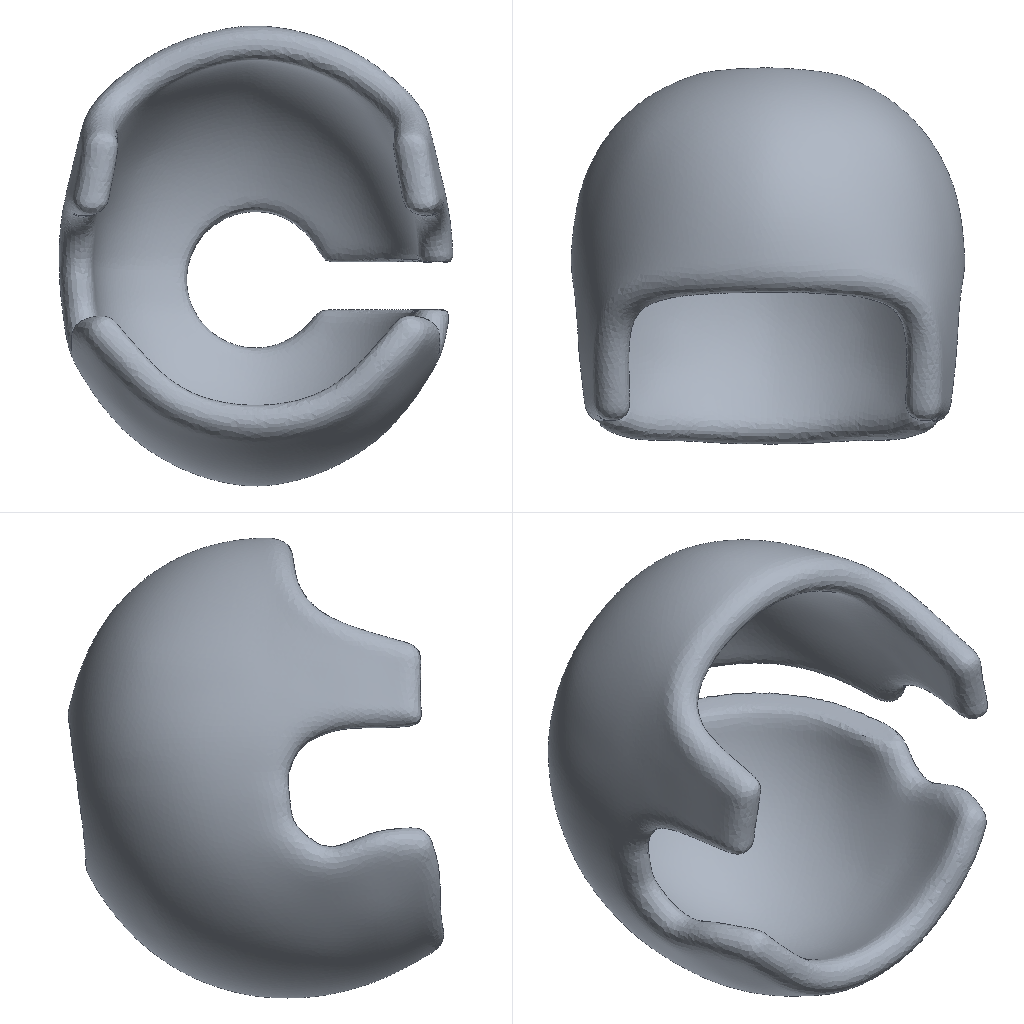Simulation study | ansys workbench
Set-up summary:
category,name,step,type,value,unit,region
solver,ansys_workbench
units,mm-N-s-tonne (MPa),,stated,"/units,MPA"
analysis,LS1,,static
load_step,LS1,LS1,static,nsubst=1; time=1
mesh,nodes,,,310599
mesh,elements,,,189958
element_type,SOLID187,,,183716
element_type,SURF154,,,6242
material,ABS?,,E,1800,tonne s^-2 mm^-1
material,ABS?,,nu,0.39
material,ABS?,,density,1.1e-09,tonne mm^-3
load,Define Force Using Surface Effect Elements,LS1,surface-effect pres face 3,0.04219,,SURF154 #2
bc,Constant Zero Displacement X,model,fixed,[dofs=UX],,_DISPZEROUX
bc,Constant Zero Displacement Y,model,fixed,[dofs=UY],,_DISPZEROUY
bc,Constant Zero Displacement Z,model,fixed,[dofs=UZ],,_DISPZEROUZ
named_set,_DISPZEROUX,,node,58563
named_set,_DISPZEROUY,,node,58563
named_set,_DISPZEROUZ,,node,58563
Ansys APDL input file, long lists of numbers shortened:
/batch
/config,noeldb,1     ! force off writing results to database
*get,_wallstrt,active,,time,wall
! ANSYS input file written by Workbench version 2022 R2
! File used for geometry attach:
/title,_____--____ (A5)
! ****** Begin Custom Load Command Snippet ******
/COM, ACT Extensions:
/COM,     LSDYNA, 2022.2
/COM,/COM,     ANSYSMotion, 2022.2
/COM,
! ****** End   Custom Load Command Snippet ******
*DIM,_wb_ProjectScratch_dir,string,248
_wb_ProjectScratch_dir(1) = ''
*DIM,_wb_SolverFiles_dir,string,248
_wb_SolverFiles_dir(1) = ''
*DIM,_wb_userfiles_dir,string,248
_wb_userfiles_dir(1) = ''
/com,--- Data in consistent NMM units. See Solving Units in the help system for more information.
/units,MPA
/nopr
/wb,file,start              !  signify a WB generated input file
/prep7
! Turn off shape checking because checks already performed inside WB mesher.
! See help system for more information.
SHPP,OFF,,NOWARN
/nolist
etcon,set             ! allow ANSYS to choose best KEYOP's for 180x elements, resets any applicable keyopt to MAPDL defaults
/com,*********** Nodes for the whole assembly ***********
nblock,3,,341658
(1i9,3e20.9e3)
        1     7.065453288E+01     2.467524350E+01     5.055699537E+02
! (310598 more lines like these left out)
-1
/wb,elem,start            !  set before creation of elements
/com,*********** Elements for Body 1 "__-FreeParts|1" ***********
et,1,187
eblock,19,solid,,183716
(19i9)
        1        1        1        1        0        0        0        0       10        0        1    35356    36573    47700    37654   265726   276079   265732   265727
! (367431 more lines like these left out)
-1
/wb,elem,end               !  done creating elements
/com,*********** Send User Defined Coordinate System(s) ***********
csys,0
toffst,273.15,  ! Temperature offset from absolute zero
/com,*********** Set Reference Temperature ***********
tref,22.
/wb,mat,start              !  starting to send materials
/com,*********** Send Materials ***********
MP,DENS,1,1.1e-09,	! tonne mm^-3
MP,EX,1,1800,	! tonne s^-2 mm^-1
MP,NUXY,1,0.39,
/wb,mat,end                !  done sending materials
!************************* Model Summary ********************
!__-FreeParts|1,	ABS塑性材料,	matid,	1
!************************* End Model Summary ********************
! get the diagonal of the bounding box. Needed later for other things
*get,_xmin,node,,mnloc,x
*get,_ymin,node,,mnloc,y
*get,_zmin,node,,mnloc,z
*get,_xmax,node,,mxloc,x
*get,_ymax,node,,mxloc,y
*get,_zmax,node,,mxloc,z
_ASMDIAG=(_xmax-_xmin)*(_xmax-_xmin)+(_ymax-_ymin)*(_ymax-_ymin)+(_zmax-_zmin)*(_zmax-_zmin)
_ASMDIAG=SQRT(_ASMDIAG)
/wb,contact,start          !  starting to send contact
/wb,contact,end            !  done creating contacts
/golist
/wb,load,start             !  starting to send loads
/com,******* Constant Zero Displacement X *******
CMBLOCK,_DISPZEROUX,NODE,    58563
(8i10)
         1         2         3         4         5         6         7         8
! (7320 more lines like these left out)
cmsel,s,_DISPZEROUX
d,all,ux,0
nsel,all
/com,******* Constant Zero Displacement Y *******
CMBLOCK,_DISPZEROUY,NODE,    58563
(8i10)
         1         2         3         4         5         6         7         8
! (7320 more lines like these left out)
cmsel,s,_DISPZEROUY
d,all,uy,0
nsel,all
/com,******* Constant Zero Displacement Z *******
CMBLOCK,_DISPZEROUZ,NODE,    58563
(8i10)
         1         2         3         4         5         6         7         8
! (7320 more lines like these left out)
cmsel,s,_DISPZEROUZ
d,all,uz,0
nsel,all
/com,*********** Define Force Using Surface Effect Elements ***********
local,12,0,0.,0.,0.,0.,0.,0.
csys,0
et,2,154
eblock,10,,,6242
(15i9)
   246685        2        2        2       12    12535    12590    12548    12548   125437   125524    12548   125434
! (6241 more lines like these left out)
-1
esel,s,type,,2
keyop,2,2,1                ! Apply load in local coordinate system
keyop,2,7,1                ! Use original area so load is constant in large deformation
esel,all
/gst,on,on
fini
*get,_numnode,node,0,count
*get,_numelem,elem,0,count
*get, _MAXELEMNUM, elem, 0, NUM, MAX
*get, _MAXNODENUM, node, 0, NUM, MAX
*get, _MAXELEMTYPE, etyp, 0, NUM, MAX
*get, _MAXREALCONST, rcon, 0, NUM, MAX
/go
/wb,load,end               !  done creating loads
/com,--- Number of total nodes = %_numnode%
/com,--- Number of contact elements = 6242
/com,--- Number of spring elements = 0
/com,--- Number of bearing elements = 0
/com,--- Number of solid elements = 183716
/com,--- Number of condensed parts = 0
/com,--- Number of total elements = %_numelem%
*get,_wallbsol,active,,time,wall
/com,****************************************************************************
/com,*************************    SOLUTION       ********************************
/com,****************************************************************************
/solu
antype,0                   ! static analysis
nlgeom,on                  ! Turn on Large Deformation Effects
_thickRatio=  1     ! Ratio of thick parts in the model
eqsl,pcg,1e-8,,,,,,1
cntr,print,1               ! print out contact info and also make no initial contact an error
dmpoption,emat,no             ! Don't combine emat file for DANSYS
dmpoption,esav,no             ! Don't combine esav file for DANSYS
nldiag,cont,iter           ! print out contact info each equilibrium iteration
rescontrol,define,last,last,,dele	   ! Program Controlled
/com,****************************************************
/com,******************* SOLVE FOR LS 1 OF 1 ****************
esel,s,type,,2
nsle
sfe,all,1,pres,1,0.
sfe,all,2,pres,1,0.
sfe,all,3,pres,1,4.21870582603669e-002
nsel,all
esel,all
/nopr
/gopr
autots,on                  ! Workbench Program Controlled automatic time stepping
nsub,1,10,1                ! due to presence of general nonlinear
time,1.
outres,erase
outres,all,none
outres,nsol,all,
outres,rsol,all
outres,eangl,all
outres,etmp,all
outres,veng,all
outres,strs,all,
outres,epel,all,
outres,eppl,all,
outres,cont,all,
! *********** WB SOLVE COMMAND ***********
! check interactive state
*get,ANSINTER_,active,,int
*if,ANSINTER_,ne,0,then
/eof
*endif
solve
/com *************** Write FE CONNECTORS *********
CEWRITE,file,ce,,INTE
/com,****************************************************
/com,*************** FINISHED SOLVE FOR LS 1 *************
*get,_wallasol,active,,time,wall
/nopr
*get,_numnode,node,0,count
*get,_numelem,elem,0,count
*get, _MAXELEMNUM, elem, 0, NUM, MAX
*get, _MAXNODENUM, node, 0, NUM, MAX,,,INTERNAL
*get, _MAXELEMTYPE, etyp, 0, NUM, MAX
*get, _MAXREALCONST, rcon, 0, NUM, MAX
*get,_NSOLTHREADS,active,0,ntfs
*get,_NSOLPROCESSES,active,0,npfs
/gopr
*get,_PCGITER,active,,solu,cgiter
/post1
xmlo,ENCODING,ISO-8859-1
xmlo,parm
/xml,parm,xml
fini
/gopr
*get,_walldone,active,,time,wall
_preptime=(_wallbsol-_wallstrt)*3600
_solvtime=(_wallasol-_wallbsol)*3600
_posttime=(_walldone-_wallasol)*3600
_totaltim=(_walldone-_wallstrt)*3600
*get,_dlbratio,active,0,solu,dlbr
*get,_combtime,active,0,solu,comb
*get,_ssmode,active,0,solu,ssmm
*get,_ndofs,active,0,solu,ndof
*get,_sol_end_time,active,0,set,time
*if,_sol_end_time,eq,1.,then
/fclean				!clean distributed files
*endif
/com,--- Total number of nodes = %_numnode%
/com,--- Total number of elements = %_numelem%
/com,--- Element load balance ratio = %_dlbratio%
/com,--- Time to combine distributed files = %_combtime%
/com,--- Sparse memory mode = %_ssmode%
/com,--- Number of DOF = %_ndofs%
/wb,file,end               ! done with WB generated input
Results summary:
result,analyses[0].index,,,1
result,analyses[0].system,,,SYS
result,analyses[0].deck,,,deck.dat
result,analyses[0].solve_status,,,completed
result,analyses[0].analysis_type,,,static
result,analyses[0].physics,,,mechanical
result,analyses[0].unit_system,,,"NMM: mm, ton, N, s, mV, mA, degC"
result,analyses[0].n_sets,,,1
result,analyses[0].load_steps[0].set,set=1,,1
result,analyses[0].load_steps[0].time_or_freq,set=1,,1
result,analyses[0].load_steps[0].max_displacement_magnitude,set=1,,0.0005219
result,analyses[0].load_steps[0].max_von_mises_nodal,set=1,,0.2653
result,analyses[0].load_steps[0].reaction_force_sum_xyz[1],set=1,,1.76306e-10
result,analyses[0].load_steps[0].reaction_force_sum_xyz[2],set=1,,2.21915e-08
result,analyses[0].load_steps[0].reaction_force_sum_xyz[3],set=1,,-350